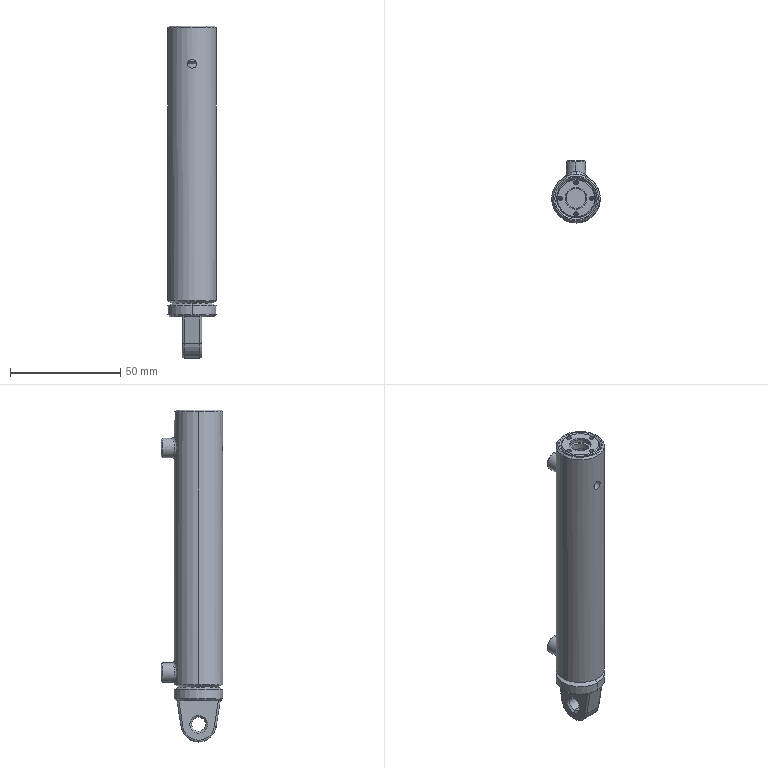Part | SolidWorks | features BaseBody 4, CombineBodies 1, Scale 1 | 1 solid | 193 faces | box 22 x 28 x 150.8 mm | volume 29606 mm3 | cylinder 87 | cone 57 | plane 35 | spline 8 | torus 6 | commonest cylinder face diameters 16 x12 1 x8 1.4 x8 2 x8 4 x6 8.96 x6